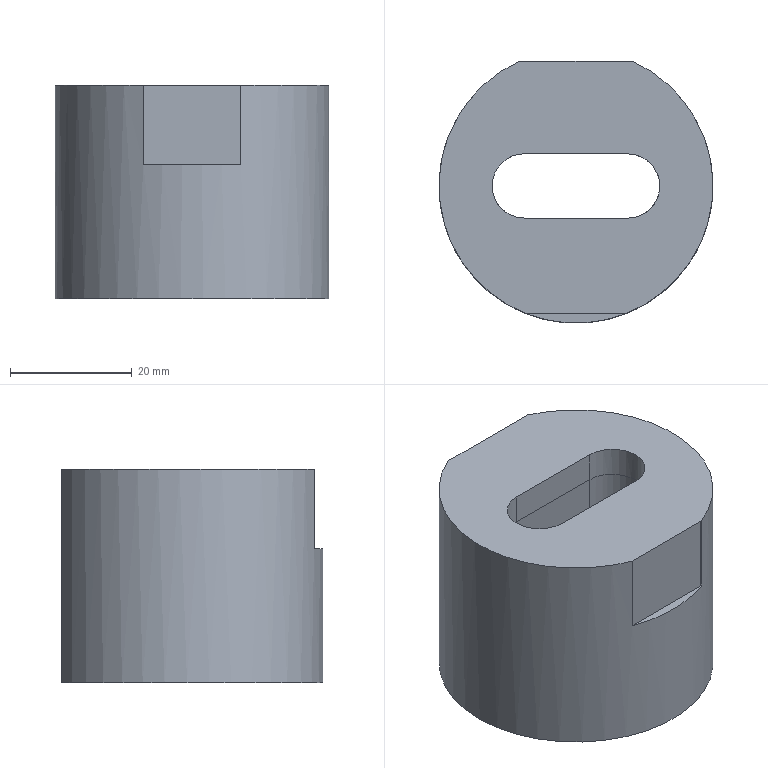Part | STEP file | lll_id322_x_t | 1 solid | 16 faces | box 45 x 43 x 35 mm | volume 44411 mm3 | plane 11 | spline 4 | cylinder 1 | commonest cylinder face diameters 45 x1
STEP:
#1=CARTESIAN_POINT('',(3410.226,-36.5,-35.));
#2=VERTEX_POINT('',#1);
#3=CARTESIAN_POINT('',(3428.774,-36.5,-35.));
#4=VERTEX_POINT('',#3);
#5=CARTESIAN_POINT('',(3419.5,-36.5,-35.));
#6=DIRECTION('',(1.,0.,0.));
#7=VECTOR('',#6,1.);
#8=LINE('',#5,#7);
#9=EDGE_CURVE('',#2,#4,#8,.T.);
#10=ORIENTED_EDGE('',*,*,#9,.T.);
#11=CARTESIAN_POINT('',(3419.5,-57.,-35.));
#12=DIRECTION('',(0.,0.,-1.));
#13=DIRECTION('',(-1.,0.,0.));
#14=AXIS2_PLACEMENT_3D('',#11,#12,#13);
#15=CIRCLE('',#14,22.5);
#16=EDGE_CURVE('',#4,#2,#15,.T.);
#17=ORIENTED_EDGE('',*,*,#16,.T.);
#18=EDGE_LOOP('',(#10,#17));
#19=FACE_BOUND('',#18,.T.);
#20=CARTESIAN_POINT('',(3411.,-63.071,-35.));
#21=VERTEX_POINT('',#20);
#22=CARTESIAN_POINT('',(3428.,-63.071,-35.));
#23=VERTEX_POINT('',#22);
#24=CARTESIAN_POINT('',(3419.5,-63.071,-35.));
#25=DIRECTION('',(1.,0.,0.));
#26=VECTOR('',#25,1.);
#27=LINE('',#24,#26);
#28=EDGE_CURVE('',#21,#23,#27,.T.);
#29=ORIENTED_EDGE('',*,*,#28,.T.);
#30=CARTESIAN_POINT('',(3428.,-50.929,-35.));
#31=VERTEX_POINT('',#30);
#32=CARTESIAN_POINT('',(3428.,-63.071,-35.));
#33=CARTESIAN_POINT('',(3428.,-63.071,-35.));
#34=CARTESIAN_POINT('',(3428.,-63.071,-35.));
#35=CARTESIAN_POINT('',(3429.609,-63.07,-35.));
#36=CARTESIAN_POINT('',(3431.162,-62.426,-35.));
#37=CARTESIAN_POINT('',(3433.432,-60.15,-35.));
#38=CARTESIAN_POINT('',(3434.072,-58.586,-35.));
#39=CARTESIAN_POINT('',(3434.069,-55.403,-35.));
#40=CARTESIAN_POINT('',(3433.419,-53.834,-35.));
#41=CARTESIAN_POINT('',(3431.167,-51.581,-35.));
#42=CARTESIAN_POINT('',(3429.612,-50.93,-35.));
#43=CARTESIAN_POINT('',(3428.,-50.929,-35.));
#44=B_SPLINE_CURVE_WITH_KNOTS('',3,(#32,#33,#34,#35,#36,#37,#38,#39,#40,#41,#42,#43),.UNSPECIFIED.,.F.,.F.,(4,2,2,2,2,4),(0.,0.00001007,0.25,0.5,0.75,1.),.UNSPECIFIED.);
#45=EDGE_CURVE('',#23,#31,#44,.T.);
#46=ORIENTED_EDGE('',*,*,#45,.T.);
#47=CARTESIAN_POINT('',(3411.,-50.929,-35.));
#48=VERTEX_POINT('',#47);
#49=CARTESIAN_POINT('',(3419.5,-50.929,-35.));
#50=DIRECTION('',(-1.,0.,0.));
#51=VECTOR('',#50,1.);
#52=LINE('',#49,#51);
#53=EDGE_CURVE('',#31,#48,#52,.T.);
#54=ORIENTED_EDGE('',*,*,#53,.T.);
#55=CARTESIAN_POINT('',(3411.,-50.929,-35.));
#56=CARTESIAN_POINT('',(3411.,-50.929,-35.));
#57=CARTESIAN_POINT('',(3411.,-50.929,-35.));
#58=CARTESIAN_POINT('',(3409.391,-50.93,-35.));
#59=CARTESIAN_POINT('',(3407.839,-51.574,-35.));
#60=CARTESIAN_POINT('',(3405.568,-53.849,-35.));
#61=CARTESIAN_POINT('',(3404.928,-55.413,-35.));
#62=CARTESIAN_POINT('',(3404.931,-58.597,-35.));
#63=CARTESIAN_POINT('',(3405.581,-60.165,-35.));
#64=CARTESIAN_POINT('',(3407.833,-62.418,-35.));
#65=CARTESIAN_POINT('',(3409.387,-63.07,-35.));
#66=CARTESIAN_POINT('',(3411.,-63.071,-35.));
#67=B_SPLINE_CURVE_WITH_KNOTS('',3,(#55,#56,#57,#58,#59,#60,#61,#62,#63,#64,#65,#66),.UNSPECIFIED.,.F.,.F.,(4,2,2,2,2,4),(0.,0.00001007,0.25,0.5,0.75,1.),.UNSPECIFIED.);
#68=EDGE_CURVE('',#48,#21,#67,.T.);
#69=ORIENTED_EDGE('',*,*,#68,.T.);
#70=EDGE_LOOP('',(#29,#46,#54,#69));
#71=FACE_BOUND('',#70,.T.);
#72=CARTESIAN_POINT('',(3419.5,-62.5,-35.));
#73=DIRECTION('',(0.,0.,-1.));
#74=DIRECTION('',(0.,1.,0.));
#75=AXIS2_PLACEMENT_3D('',#72,#73,#74);
#76=PLANE('',#75);
#77=ADVANCED_FACE('',(#19,#71),#76,.T.);
#78=CARTESIAN_POINT('',(3427.5,-78.,0.00001771));
#79=VERTEX_POINT('',#78);
#80=CARTESIAN_POINT('',(3411.5,-78.,0.00001771));
#81=VERTEX_POINT('',#80);
#82=CARTESIAN_POINT('',(3419.5,-78.,0.00001771));
#83=DIRECTION('',(-1.,0.,0.));
#84=VECTOR('',#83,1.);
#85=LINE('',#82,#84);
#86=EDGE_CURVE('',#79,#81,#85,.T.);
#87=ORIENTED_EDGE('',*,*,#86,.F.);
#88=CARTESIAN_POINT('',(3427.5,-78.03,0.00001771));
#89=VERTEX_POINT('',#88);
#90=CARTESIAN_POINT('',(3427.5,-86.,0.00001771));
#91=DIRECTION('',(0.,-1.,0.));
#92=VECTOR('',#91,1.);
#93=LINE('',#90,#92);
#94=EDGE_CURVE('',#79,#89,#93,.T.);
#95=ORIENTED_EDGE('',*,*,#94,.T.);
#96=CARTESIAN_POINT('',(3428.774,-36.5,0.00001771));
#97=VERTEX_POINT('',#96);
#98=CARTESIAN_POINT('',(3419.5,-57.,0.00001771));
#99=DIRECTION('',(0.,0.,-1.));
#100=DIRECTION('',(-1.,0.,0.));
#101=AXIS2_PLACEMENT_3D('',#98,#99,#100);
#102=CIRCLE('',#101,22.5);
#103=EDGE_CURVE('',#97,#89,#102,.T.);
#104=ORIENTED_EDGE('',*,*,#103,.F.);
#105=CARTESIAN_POINT('',(3410.226,-36.5,0.00001771));
#106=VERTEX_POINT('',#105);
#107=CARTESIAN_POINT('',(3419.5,-36.5,0.00001771));
#108=DIRECTION('',(-1.,0.,0.));
#109=VECTOR('',#108,1.);
#110=LINE('',#107,#109);
#111=EDGE_CURVE('',#97,#106,#110,.T.);
#112=ORIENTED_EDGE('',*,*,#111,.T.);
#113=CARTESIAN_POINT('',(3411.5,-78.03,0.00001771));
#114=VERTEX_POINT('',#113);
#115=CARTESIAN_POINT('',(3419.5,-57.,0.00001771));
#116=DIRECTION('',(0.,0.,-1.));
#117=DIRECTION('',(-1.,0.,0.));
#118=AXIS2_PLACEMENT_3D('',#115,#116,#117);
#119=CIRCLE('',#118,22.5);
#120=EDGE_CURVE('',#114,#106,#119,.T.);
#121=ORIENTED_EDGE('',*,*,#120,.F.);
#122=CARTESIAN_POINT('',(3411.5,-57.,0.00001771));
#123=DIRECTION('',(0.,-1.,0.));
#124=VECTOR('',#123,1.);
#125=LINE('',#122,#124);
#126=EDGE_CURVE('',#81,#114,#125,.T.);
#127=ORIENTED_EDGE('',*,*,#126,.F.);
#128=EDGE_LOOP('',(#87,#95,#104,#112,#121,#127));
#129=FACE_BOUND('',#128,.T.);
#130=CARTESIAN_POINT('',(3428.,-51.715,0.00001771));
#131=VERTEX_POINT('',#130);
#132=CARTESIAN_POINT('',(3428.,-62.285,0.00001771));
#133=VERTEX_POINT('',#132);
#134=CARTESIAN_POINT('',(3428.,-51.715,0.00001769));
#135=CARTESIAN_POINT('',(3429.386,-51.715,0.0000177));
#136=CARTESIAN_POINT('',(3430.756,-52.282,0.00001771));
#137=CARTESIAN_POINT('',(3432.718,-54.244,0.00001773));
#138=CARTESIAN_POINT('',(3433.285,-55.613,0.00001773));
#139=CARTESIAN_POINT('',(3433.285,-58.387,0.00001773));
#140=CARTESIAN_POINT('',(3432.718,-59.756,0.00001773));
#141=CARTESIAN_POINT('',(3431.247,-61.227,0.00001772));
#142=CARTESIAN_POINT('',(3430.659,-61.614,0.00001771));
#143=CARTESIAN_POINT('',(3429.701,-62.01,0.0000177));
#144=CARTESIAN_POINT('',(3429.37,-62.112,0.0000177));
#145=CARTESIAN_POINT('',(3428.692,-62.249,0.0000177));
#146=CARTESIAN_POINT('',(3428.33,-62.285,0.00001769));
#147=CARTESIAN_POINT('',(3428.,-62.285,0.00001769));
#148=B_SPLINE_CURVE_WITH_KNOTS('',3,(#134,#135,#136,#137,#138,#139,#140,#141,#142,#143,#144,#145,#146,#147),.UNSPECIFIED.,.F.,.F.,(4,2,2,2,2,2,4),(0.,0.25,0.5,0.75,0.875,0.9375,1.),.UNSPECIFIED.);
#149=EDGE_CURVE('',#131,#133,#148,.T.);
#150=ORIENTED_EDGE('',*,*,#149,.T.);
#151=CARTESIAN_POINT('',(3411.,-62.285,0.00001771));
#152=VERTEX_POINT('',#151);
#153=CARTESIAN_POINT('',(3419.5,-62.285,0.00001771));
#154=DIRECTION('',(-1.,0.,0.));
#155=VECTOR('',#154,1.);
#156=LINE('',#153,#155);
#157=EDGE_CURVE('',#133,#152,#156,.T.);
#158=ORIENTED_EDGE('',*,*,#157,.T.);
#159=CARTESIAN_POINT('',(3411.,-51.715,0.00001771));
#160=VERTEX_POINT('',#159);
#161=CARTESIAN_POINT('',(3411.,-62.285,0.00001772));
#162=CARTESIAN_POINT('',(3409.622,-62.285,0.00001771));
#163=CARTESIAN_POINT('',(3408.244,-61.719,0.0000177));
#164=CARTESIAN_POINT('',(3406.282,-59.756,0.00001769));
#165=CARTESIAN_POINT('',(3405.715,-58.387,0.00001768));
#166=CARTESIAN_POINT('',(3405.715,-55.613,0.00001768));
#167=CARTESIAN_POINT('',(3406.282,-54.244,0.00001769));
#168=CARTESIAN_POINT('',(3408.244,-52.282,0.0000177));
#169=CARTESIAN_POINT('',(3409.613,-51.715,0.00001771));
#170=CARTESIAN_POINT('',(3411.,-51.715,0.00001772));
#171=B_SPLINE_CURVE_WITH_KNOTS('',3,(#161,#162,#163,#164,#165,#166,#167,#168,#169,#170),.UNSPECIFIED.,.F.,.F.,(4,2,2,2,4),(0.,0.25,0.5,0.75,1.),.UNSPECIFIED.);
#172=EDGE_CURVE('',#152,#160,#171,.T.);
#173=ORIENTED_EDGE('',*,*,#172,.T.);
#174=CARTESIAN_POINT('',(3419.5,-51.715,0.00001771));
#175=DIRECTION('',(1.,0.,0.));
#176=VECTOR('',#175,1.);
#177=LINE('',#174,#176);
#178=EDGE_CURVE('',#160,#131,#177,.T.);
#179=ORIENTED_EDGE('',*,*,#178,.T.);
#180=EDGE_LOOP('',(#150,#158,#173,#179));
#181=FACE_BOUND('',#180,.T.);
#182=CARTESIAN_POINT('',(3419.5,-57.,0.00001771));
#183=DIRECTION('',(0.,0.,1.));
#184=DIRECTION('',(1.,0.,0.));
#185=AXIS2_PLACEMENT_3D('',#182,#183,#184);
#186=PLANE('',#185);
#187=ADVANCED_FACE('',(#129,#181),#186,.T.);
#188=ORIENTED_EDGE('',*,*,#103,.T.);
#189=CARTESIAN_POINT('',(3427.5,-78.03,-13.));
#190=VERTEX_POINT('',#189);
#191=CARTESIAN_POINT('',(3427.5,-78.03,-15.));
#192=DIRECTION('',(0.,0.,1.));
#193=VECTOR('',#192,1.);
#194=LINE('',#191,#193);
#195=EDGE_CURVE('',#190,#89,#194,.T.);
#196=ORIENTED_EDGE('',*,*,#195,.F.);
#197=CARTESIAN_POINT('',(3411.5,-78.03,-13.));
#198=VERTEX_POINT('',#197);
#199=CARTESIAN_POINT('',(3419.5,-57.,-13.));
#200=DIRECTION('',(0.,0.,1.));
#201=DIRECTION('',(-1.,0.,0.));
#202=AXIS2_PLACEMENT_3D('',#199,#200,#201);
#203=CIRCLE('',#202,22.5);
#204=EDGE_CURVE('',#198,#190,#203,.T.);
#205=ORIENTED_EDGE('',*,*,#204,.F.);
#206=CARTESIAN_POINT('',(3411.5,-78.03,-15.));
#207=DIRECTION('',(0.,0.,-1.));
#208=VECTOR('',#207,1.);
#209=LINE('',#206,#208);
#210=EDGE_CURVE('',#114,#198,#209,.T.);
#211=ORIENTED_EDGE('',*,*,#210,.F.);
#212=ORIENTED_EDGE('',*,*,#120,.T.);
#213=CARTESIAN_POINT('',(3410.226,-36.5,-15.));
#214=DIRECTION('',(0.,0.,-1.));
#215=VECTOR('',#214,1.);
#216=LINE('',#213,#215);
#217=EDGE_CURVE('',#106,#2,#216,.T.);
#218=ORIENTED_EDGE('',*,*,#217,.T.);
#219=ORIENTED_EDGE('',*,*,#16,.F.);
#220=CARTESIAN_POINT('',(3428.774,-36.5,-15.));
#221=DIRECTION('',(0.,0.,1.));
#222=VECTOR('',#221,1.);
#223=LINE('',#220,#222);
#224=EDGE_CURVE('',#4,#97,#223,.T.);
#225=ORIENTED_EDGE('',*,*,#224,.T.);
#226=EDGE_LOOP('',(#188,#196,#205,#211,#212,#218,#219,#225));
#227=FACE_OUTER_BOUND('',#226,.T.);
#228=CARTESIAN_POINT('',(3419.5,-57.,-15.));
#229=DIRECTION('',(0.,0.,-1.));
#230=DIRECTION('',(0.,-1.,0.));
#231=AXIS2_PLACEMENT_3D('',#228,#229,#230);
#232=CYLINDRICAL_SURFACE('',#231,22.5);
#233=ADVANCED_FACE('',(#227),#232,.T.);
#234=CARTESIAN_POINT('',(3428.,-62.285,-5.));
#235=VERTEX_POINT('',#234);
#236=CARTESIAN_POINT('',(3411.,-62.285,-5.));
#237=VERTEX_POINT('',#236);
#238=CARTESIAN_POINT('',(3428.,-62.285,-5.));
#239=DIRECTION('',(-1.,0.,0.));
#240=VECTOR('',#239,1.);
#241=LINE('',#238,#240);
#242=EDGE_CURVE('',#235,#237,#241,.T.);
#243=ORIENTED_EDGE('',*,*,#242,.T.);
#244=CARTESIAN_POINT('',(3411.,-62.285,2.5));
#245=DIRECTION('',(-0.000000008,0.,1.));
#246=VECTOR('',#245,1.);
#247=LINE('',#244,#246);
#248=EDGE_CURVE('',#237,#152,#247,.T.);
#249=ORIENTED_EDGE('',*,*,#248,.T.);
#250=ORIENTED_EDGE('',*,*,#157,.F.);
#251=CARTESIAN_POINT('',(3428.,-62.285,2.5));
#252=DIRECTION('',(-0.000000008,0.,1.));
#253=VECTOR('',#252,1.);
#254=LINE('',#251,#253);
#255=EDGE_CURVE('',#235,#133,#254,.T.);
#256=ORIENTED_EDGE('',*,*,#255,.F.);
#257=EDGE_LOOP('',(#243,#249,#250,#256));
#258=FACE_OUTER_BOUND('',#257,.T.);
#259=CARTESIAN_POINT('',(3433.,-62.285,2.5));
#260=DIRECTION('',(0.,1.,0.));
#261=DIRECTION('',(-1.,0.,-0.000000008));
#262=AXIS2_PLACEMENT_3D('',#259,#260,#261);
#263=PLANE('',#262);
#264=ADVANCED_FACE('',(#258),#263,.T.);
#265=CARTESIAN_POINT('',(3428.005,-62.285,-5.));
#266=VERTEX_POINT('',#265);
#267=CARTESIAN_POINT('',(3428.005,-62.285,-5.));
#268=CARTESIAN_POINT('',(3428.004,-62.285,-5.));
#269=CARTESIAN_POINT('',(3428.002,-62.285,-5.));
#270=CARTESIAN_POINT('',(3428.,-62.285,-5.));
#271=B_SPLINE_CURVE_WITH_KNOTS('',3,(#267,#268,#269,#270),.UNSPECIFIED.,.F.,.F.,(4,4),(0.,1.),.UNSPECIFIED.);
#272=EDGE_CURVE('',#266,#235,#271,.T.);
#273=ORIENTED_EDGE('',*,*,#272,.T.);
#274=ORIENTED_EDGE('',*,*,#255,.T.);
#275=ORIENTED_EDGE('',*,*,#149,.F.);
#276=CARTESIAN_POINT('',(3428.,-51.715,-5.));
#277=VERTEX_POINT('',#276);
#278=CARTESIAN_POINT('',(3428.,-51.715,2.5));
#279=DIRECTION('',(-0.000000008,0.,1.));
#280=VECTOR('',#279,1.);
#281=LINE('',#278,#280);
#282=EDGE_CURVE('',#277,#131,#281,.T.);
#283=ORIENTED_EDGE('',*,*,#282,.F.);
#284=CARTESIAN_POINT('',(3428.006,-51.715,-5.));
#285=VERTEX_POINT('',#284);
#286=CARTESIAN_POINT('',(3428.,-51.715,-5.));
#287=CARTESIAN_POINT('',(3428.002,-51.715,-5.));
#288=CARTESIAN_POINT('',(3428.004,-51.715,-5.));
#289=CARTESIAN_POINT('',(3428.006,-51.715,-5.));
#290=B_SPLINE_CURVE_WITH_KNOTS('',3,(#286,#287,#288,#289),.UNSPECIFIED.,.F.,.F.,(4,4),(0.,1.),.UNSPECIFIED.);
#291=EDGE_CURVE('',#277,#285,#290,.T.);
#292=ORIENTED_EDGE('',*,*,#291,.T.);
#293=CARTESIAN_POINT('',(3431.732,-53.258,-5.));
#294=VERTEX_POINT('',#293);
#295=CARTESIAN_POINT('',(3428.006,-51.715,-5.));
#296=CARTESIAN_POINT('',(3429.388,-51.717,-5.));
#297=CARTESIAN_POINT('',(3430.753,-52.282,-5.));
#298=CARTESIAN_POINT('',(3431.732,-53.258,-5.));
#299=B_SPLINE_CURVE_WITH_KNOTS('',3,(#295,#296,#297,#298),.UNSPECIFIED.,.F.,.F.,(4,4),(0.,1.),.UNSPECIFIED.);
#300=EDGE_CURVE('',#285,#294,#299,.T.);
#301=ORIENTED_EDGE('',*,*,#300,.T.);
#302=CARTESIAN_POINT('',(3433.285,-56.998,-5.));
#303=VERTEX_POINT('',#302);
#304=CARTESIAN_POINT('',(3431.732,-53.258,-5.));
#305=CARTESIAN_POINT('',(3431.896,-53.421,-5.));
#306=CARTESIAN_POINT('',(3432.133,-53.675,-5.012));
#307=CARTESIAN_POINT('',(3432.645,-54.445,-5.058));
#308=CARTESIAN_POINT('',(3432.789,-54.762,-5.07));
#309=CARTESIAN_POINT('',(3432.965,-55.188,-5.07));
#310=CARTESIAN_POINT('',(3433.089,-55.513,-5.059));
#311=CARTESIAN_POINT('',(3433.272,-56.419,-5.012));
#312=CARTESIAN_POINT('',(3433.285,-56.768,-5.));
#313=CARTESIAN_POINT('',(3433.285,-56.998,-5.));
#314=B_SPLINE_CURVE_WITH_KNOTS('',3,(#304,#305,#306,#307,#308,#309,#310,#311,#312,#313),.UNSPECIFIED.,.F.,.F.,(4,2,2,2,4),(0.,0.25,0.5,0.75,1.),.UNSPECIFIED.);
#315=EDGE_CURVE('',#294,#303,#314,.T.);
#316=ORIENTED_EDGE('',*,*,#315,.T.);
#317=CARTESIAN_POINT('',(3433.045,-58.562,-5.));
#318=VERTEX_POINT('',#317);
#319=CARTESIAN_POINT('',(3433.285,-56.998,-5.001));
#320=CARTESIAN_POINT('',(3433.285,-56.998,-5.001));
#321=CARTESIAN_POINT('',(3433.285,-56.999,-5.001));
#322=CARTESIAN_POINT('',(3433.285,-57.53,-5.001));
#323=CARTESIAN_POINT('',(3433.202,-58.058,-5.001));
#324=CARTESIAN_POINT('',(3433.045,-58.562,-5.001));
#325=B_SPLINE_CURVE_WITH_KNOTS('',3,(#319,#320,#321,#322,#323,#324),.UNSPECIFIED.,.F.,.F.,(4,2,4),(0.,0.001523,1.),.UNSPECIFIED.);
#326=EDGE_CURVE('',#303,#318,#325,.T.);
#327=ORIENTED_EDGE('',*,*,#326,.T.);
#328=CARTESIAN_POINT('',(3431.742,-60.732,-5.));
#329=VERTEX_POINT('',#328);
#330=CARTESIAN_POINT('',(3433.045,-58.562,-5.));
#331=CARTESIAN_POINT('',(3432.792,-59.375,-5.));
#332=CARTESIAN_POINT('',(3432.346,-60.127,-5.));
#333=CARTESIAN_POINT('',(3431.742,-60.732,-5.));
#334=B_SPLINE_CURVE_WITH_KNOTS('',3,(#330,#331,#332,#333),.UNSPECIFIED.,.F.,.F.,(4,4),(0.,1.),.UNSPECIFIED.);
#335=EDGE_CURVE('',#318,#329,#334,.T.);
#336=ORIENTED_EDGE('',*,*,#335,.T.);
#337=CARTESIAN_POINT('',(3431.742,-60.732,-5.));
#338=CARTESIAN_POINT('',(3431.741,-60.734,-5.));
#339=CARTESIAN_POINT('',(3431.739,-60.735,-5.));
#340=CARTESIAN_POINT('',(3431.247,-61.227,-5.));
#341=CARTESIAN_POINT('',(3430.659,-61.614,-5.));
#342=CARTESIAN_POINT('',(3429.701,-62.01,-5.));
#343=CARTESIAN_POINT('',(3429.37,-62.112,-5.));
#344=CARTESIAN_POINT('',(3428.694,-62.249,-5.));
#345=CARTESIAN_POINT('',(3428.334,-62.285,-5.));
#346=CARTESIAN_POINT('',(3428.005,-62.285,-5.));
#347=B_SPLINE_CURVE_WITH_KNOTS('',3,(#337,#338,#339,#340,#341,#342,#343,#344,#345,#346),.UNSPECIFIED.,.F.,.F.,(4,2,2,2,4),(0.,0.001784,0.5016,0.7515,1.),.UNSPECIFIED.);
#348=EDGE_CURVE('',#329,#266,#347,.T.);
#349=ORIENTED_EDGE('',*,*,#348,.T.);
#350=EDGE_LOOP('',(#273,#274,#275,#283,#292,#301,#316,#327,#336,#349));
#351=FACE_OUTER_BOUND('',#350,.T.);
#352=CARTESIAN_POINT('',(3428.,-51.715,-5.106));
#353=CARTESIAN_POINT('',(3428.,-51.715,0.00001771));
#354=CARTESIAN_POINT('',(3429.386,-51.715,-5.106));
#355=CARTESIAN_POINT('',(3429.386,-51.715,0.00001772));
#356=CARTESIAN_POINT('',(3430.756,-52.282,-5.106));
#357=CARTESIAN_POINT('',(3430.756,-52.282,0.00001773));
#358=CARTESIAN_POINT('',(3432.718,-54.244,-5.106));
#359=CARTESIAN_POINT('',(3432.718,-54.244,0.00001775));
#360=CARTESIAN_POINT('',(3433.285,-55.613,-5.106));
#361=CARTESIAN_POINT('',(3433.285,-55.613,0.00001775));
#362=CARTESIAN_POINT('',(3433.285,-58.387,-5.106));
#363=CARTESIAN_POINT('',(3433.285,-58.387,0.00001775));
#364=CARTESIAN_POINT('',(3432.718,-59.756,-5.106));
#365=CARTESIAN_POINT('',(3432.718,-59.756,0.00001775));
#366=CARTESIAN_POINT('',(3431.247,-61.227,-5.106));
#367=CARTESIAN_POINT('',(3431.247,-61.227,0.00001774));
#368=CARTESIAN_POINT('',(3430.659,-61.614,-5.106));
#369=CARTESIAN_POINT('',(3430.659,-61.614,0.00001773));
#370=CARTESIAN_POINT('',(3429.701,-62.01,-5.106));
#371=CARTESIAN_POINT('',(3429.701,-62.01,0.00001772));
#372=CARTESIAN_POINT('',(3429.37,-62.112,-5.106));
#373=CARTESIAN_POINT('',(3429.37,-62.112,0.00001772));
#374=CARTESIAN_POINT('',(3428.692,-62.249,-5.106));
#375=CARTESIAN_POINT('',(3428.692,-62.249,0.00001772));
#376=CARTESIAN_POINT('',(3428.33,-62.285,-5.106));
#377=CARTESIAN_POINT('',(3428.33,-62.285,0.00001771));
#378=CARTESIAN_POINT('',(3428.,-62.285,-5.106));
#379=CARTESIAN_POINT('',(3428.,-62.285,0.00001771));
#380=B_SPLINE_SURFACE_WITH_KNOTS('',3,1,((#352,#353),(#354,#355),(#356,#357),(#358,#359),(#360,#361),(#362,#363),(#364,#365),(#366,#367),(#368,#369),(#370,#371),(#372,#373),(#374,#375),(#376,#377),(#378,#379)),.UNSPECIFIED.,.F.,.F.,.F.,(4,2,2,2,2,2,4),(2,2),(0.,0.25,0.5,0.75,0.875,0.9375,1.),(0.,1.),.UNSPECIFIED.);
#381=ADVANCED_FACE('',(#351),#380,.T.);
#382=CARTESIAN_POINT('',(3411.,-51.715,-5.));
#383=VERTEX_POINT('',#382);
#384=CARTESIAN_POINT('',(3411.,-51.715,-5.));
#385=DIRECTION('',(1.,0.,0.));
#386=VECTOR('',#385,1.);
#387=LINE('',#384,#386);
#388=EDGE_CURVE('',#383,#277,#387,.T.);
#389=ORIENTED_EDGE('',*,*,#388,.T.);
#390=ORIENTED_EDGE('',*,*,#282,.T.);
#391=ORIENTED_EDGE('',*,*,#178,.F.);
#392=CARTESIAN_POINT('',(3411.,-51.715,2.5));
#393=DIRECTION('',(-0.000000008,0.,1.));
#394=VECTOR('',#393,1.);
#395=LINE('',#392,#394);
#396=EDGE_CURVE('',#383,#160,#395,.T.);
#397=ORIENTED_EDGE('',*,*,#396,.F.);
#398=EDGE_LOOP('',(#389,#390,#391,#397));
#399=FACE_OUTER_BOUND('',#398,.T.);
#400=CARTESIAN_POINT('',(3433.,-51.715,2.5));
#401=DIRECTION('',(0.,-1.,0.));
#402=DIRECTION('',(1.,0.,0.000000008));
#403=AXIS2_PLACEMENT_3D('',#400,#401,#402);
#404=PLANE('',#403);
#405=ADVANCED_FACE('',(#399),#404,.T.);
#406=CARTESIAN_POINT('',(3410.995,-51.715,-5.));
#407=VERTEX_POINT('',#406);
#408=CARTESIAN_POINT('',(3410.995,-51.715,-5.));
#409=CARTESIAN_POINT('',(3410.996,-51.715,-5.));
#410=CARTESIAN_POINT('',(3410.998,-51.715,-5.));
#411=CARTESIAN_POINT('',(3411.,-51.715,-5.));
#412=B_SPLINE_CURVE_WITH_KNOTS('',3,(#408,#409,#410,#411),.UNSPECIFIED.,.F.,.F.,(4,4),(0.,1.),.UNSPECIFIED.);
#413=EDGE_CURVE('',#407,#383,#412,.T.);
#414=ORIENTED_EDGE('',*,*,#413,.T.);
#415=ORIENTED_EDGE('',*,*,#396,.T.);
#416=ORIENTED_EDGE('',*,*,#172,.F.);
#417=ORIENTED_EDGE('',*,*,#248,.F.);
#418=CARTESIAN_POINT('',(3410.994,-62.285,-5.));
#419=VERTEX_POINT('',#418);
#420=CARTESIAN_POINT('',(3411.,-62.285,-5.));
#421=CARTESIAN_POINT('',(3410.998,-62.285,-5.));
#422=CARTESIAN_POINT('',(3410.996,-62.285,-5.));
#423=CARTESIAN_POINT('',(3410.994,-62.285,-5.));
#424=B_SPLINE_CURVE_WITH_KNOTS('',3,(#420,#421,#422,#423),.UNSPECIFIED.,.F.,.F.,(4,4),(0.,1.),.UNSPECIFIED.);
#425=EDGE_CURVE('',#237,#419,#424,.T.);
#426=ORIENTED_EDGE('',*,*,#425,.T.);
#427=CARTESIAN_POINT('',(3407.26,-60.734,-5.));
#428=VERTEX_POINT('',#427);
#429=CARTESIAN_POINT('',(3410.994,-62.285,-5.));
#430=CARTESIAN_POINT('',(3409.618,-62.283,-5.));
#431=CARTESIAN_POINT('',(3408.243,-61.717,-5.));
#432=CARTESIAN_POINT('',(3407.262,-60.736,-5.));
#433=CARTESIAN_POINT('',(3407.261,-60.735,-5.));
#434=CARTESIAN_POINT('',(3407.26,-60.734,-5.));
#435=B_SPLINE_CURVE_WITH_KNOTS('',3,(#429,#430,#431,#432,#433,#434),.UNSPECIFIED.,.F.,.F.,(4,2,4),(0.,0.9989,1.),.UNSPECIFIED.);
#436=EDGE_CURVE('',#419,#428,#435,.T.);
#437=ORIENTED_EDGE('',*,*,#436,.T.);
#438=CARTESIAN_POINT('',(3405.715,-57.002,-5.));
#439=VERTEX_POINT('',#438);
#440=CARTESIAN_POINT('',(3407.26,-60.734,-5.));
#441=CARTESIAN_POINT('',(3407.098,-60.572,-5.));
#442=CARTESIAN_POINT('',(3406.861,-60.316,-5.012));
#443=CARTESIAN_POINT('',(3406.352,-59.549,-5.059));
#444=CARTESIAN_POINT('',(3406.208,-59.232,-5.071));
#445=CARTESIAN_POINT('',(3406.033,-58.808,-5.071));
#446=CARTESIAN_POINT('',(3405.91,-58.483,-5.059));
#447=CARTESIAN_POINT('',(3405.728,-57.58,-5.012));
#448=CARTESIAN_POINT('',(3405.715,-57.232,-5.));
#449=CARTESIAN_POINT('',(3405.715,-57.002,-5.));
#450=B_SPLINE_CURVE_WITH_KNOTS('',3,(#440,#441,#442,#443,#444,#445,#446,#447,#448,#449),.UNSPECIFIED.,.F.,.F.,(4,2,2,2,4),(0.,0.25,0.5,0.75,1.),.UNSPECIFIED.);
#451=EDGE_CURVE('',#428,#439,#450,.T.);
#452=ORIENTED_EDGE('',*,*,#451,.T.);
#453=CARTESIAN_POINT('',(3406.035,-55.202,-5.));
#454=VERTEX_POINT('',#453);
#455=CARTESIAN_POINT('',(3405.715,-57.002,-5.001));
#456=CARTESIAN_POINT('',(3405.715,-57.002,-5.001));
#457=CARTESIAN_POINT('',(3405.715,-57.001,-5.001));
#458=CARTESIAN_POINT('',(3405.715,-56.387,-5.001));
#459=CARTESIAN_POINT('',(3405.826,-55.776,-5.001));
#460=CARTESIAN_POINT('',(3406.035,-55.202,-5.001));
#461=B_SPLINE_CURVE_WITH_KNOTS('',3,(#455,#456,#457,#458,#459,#460),.UNSPECIFIED.,.F.,.F.,(4,2,4),(0.,0.001199,1.),.UNSPECIFIED.);
#462=EDGE_CURVE('',#439,#454,#461,.T.);
#463=ORIENTED_EDGE('',*,*,#462,.T.);
#464=CARTESIAN_POINT('',(3407.258,-53.268,-5.));
#465=VERTEX_POINT('',#464);
#466=CARTESIAN_POINT('',(3406.035,-55.202,-5.));
#467=CARTESIAN_POINT('',(3406.297,-54.48,-5.));
#468=CARTESIAN_POINT('',(3406.713,-53.814,-5.));
#469=CARTESIAN_POINT('',(3407.258,-53.268,-5.));
#470=B_SPLINE_CURVE_WITH_KNOTS('',3,(#466,#467,#468,#469),.UNSPECIFIED.,.F.,.F.,(4,4),(0.,1.),.UNSPECIFIED.);
#471=EDGE_CURVE('',#454,#465,#470,.T.);
#472=ORIENTED_EDGE('',*,*,#471,.T.);
#473=CARTESIAN_POINT('',(3407.258,-53.268,-5.));
#474=CARTESIAN_POINT('',(3407.259,-53.266,-5.));
#475=CARTESIAN_POINT('',(3407.261,-53.265,-5.));
#476=CARTESIAN_POINT('',(3408.242,-52.283,-5.));
#477=CARTESIAN_POINT('',(3409.61,-51.717,-5.));
#478=CARTESIAN_POINT('',(3410.995,-51.715,-5.));
#479=B_SPLINE_CURVE_WITH_KNOTS('',3,(#473,#474,#475,#476,#477,#478),.UNSPECIFIED.,.F.,.F.,(4,2,4),(0.,0.001796,1.),.UNSPECIFIED.);
#480=EDGE_CURVE('',#465,#407,#479,.T.);
#481=ORIENTED_EDGE('',*,*,#480,.T.);
#482=EDGE_LOOP('',(#414,#415,#416,#417,#426,#437,#452,#463,#472,#481));
#483=FACE_OUTER_BOUND('',#482,.T.);
#484=CARTESIAN_POINT('',(3411.,-62.285,-5.108));
#485=CARTESIAN_POINT('',(3411.,-62.285,0.00001773));
#486=CARTESIAN_POINT('',(3409.622,-62.285,-5.108));
#487=CARTESIAN_POINT('',(3409.622,-62.285,0.00001772));
#488=CARTESIAN_POINT('',(3408.244,-61.719,-5.108));
#489=CARTESIAN_POINT('',(3408.244,-61.719,0.00001771));
#490=CARTESIAN_POINT('',(3406.282,-59.756,-5.108));
#491=CARTESIAN_POINT('',(3406.282,-59.756,0.0000177));
#492=CARTESIAN_POINT('',(3405.715,-58.387,-5.108));
#493=CARTESIAN_POINT('',(3405.715,-58.387,0.00001769));
#494=CARTESIAN_POINT('',(3405.715,-55.613,-5.108));
#495=CARTESIAN_POINT('',(3405.715,-55.613,0.00001769));
#496=CARTESIAN_POINT('',(3406.282,-54.244,-5.108));
#497=CARTESIAN_POINT('',(3406.282,-54.244,0.0000177));
#498=CARTESIAN_POINT('',(3408.244,-52.282,-5.108));
#499=CARTESIAN_POINT('',(3408.244,-52.282,0.00001771));
#500=CARTESIAN_POINT('',(3409.613,-51.715,-5.108));
#501=CARTESIAN_POINT('',(3409.613,-51.715,0.00001772));
#502=CARTESIAN_POINT('',(3411.,-51.715,-5.108));
#503=CARTESIAN_POINT('',(3411.,-51.715,0.00001773));
#504=B_SPLINE_SURFACE_WITH_KNOTS('',3,1,((#484,#485),(#486,#487),(#488,#489),(#490,#491),(#492,#493),(#494,#495),(#496,#497),(#498,#499),(#500,#501),(#502,#503)),.UNSPECIFIED.,.F.,.F.,.F.,(4,2,2,2,4),(2,2),(0.,0.25,0.5,0.75,1.),(0.,1.),.UNSPECIFIED.);
#505=ADVANCED_FACE('',(#483),#504,.T.);
#506=ORIENTED_EDGE('',*,*,#224,.F.);
#507=ORIENTED_EDGE('',*,*,#9,.F.);
#508=ORIENTED_EDGE('',*,*,#217,.F.);
#509=ORIENTED_EDGE('',*,*,#111,.F.);
#510=EDGE_LOOP('',(#506,#507,#508,#509));
#511=FACE_OUTER_BOUND('',#510,.T.);
#512=CARTESIAN_POINT('',(3419.5,-36.5,-32.5));
#513=DIRECTION('',(0.,1.,0.));
#514=DIRECTION('',(0.,0.,-1.));
#515=AXIS2_PLACEMENT_3D('',#512,#513,#514);
#516=PLANE('',#515);
#517=ADVANCED_FACE('',(#511),#516,.T.);
#518=CARTESIAN_POINT('',(3428.,-62.285,-5.));
#519=DIRECTION('',(0.,-0.02618,-0.9997));
#520=VECTOR('',#519,1.);
#521=LINE('',#518,#520);
#522=EDGE_CURVE('',#235,#23,#521,.T.);
#523=ORIENTED_EDGE('',*,*,#522,.F.);
#524=ORIENTED_EDGE('',*,*,#272,.F.);
#525=ORIENTED_EDGE('',*,*,#348,.F.);
#526=ORIENTED_EDGE('',*,*,#335,.F.);
#527=ORIENTED_EDGE('',*,*,#326,.F.);
#528=ORIENTED_EDGE('',*,*,#315,.F.);
#529=ORIENTED_EDGE('',*,*,#300,.F.);
#530=ORIENTED_EDGE('',*,*,#291,.F.);
#531=CARTESIAN_POINT('',(3428.,-51.715,-5.));
#532=DIRECTION('',(0.000006156,0.02618,-0.9997));
#533=VECTOR('',#532,1.);
#534=LINE('',#531,#533);
#535=EDGE_CURVE('',#277,#31,#534,.T.);
#536=ORIENTED_EDGE('',*,*,#535,.T.);
#537=ORIENTED_EDGE('',*,*,#45,.F.);
#538=EDGE_LOOP('',(#523,#524,#525,#526,#527,#528,#529,#530,#536,#537));
#539=FACE_OUTER_BOUND('',#538,.T.);
#540=CARTESIAN_POINT('',(3428.,-51.715,-5.));
#541=CARTESIAN_POINT('',(3429.396,-51.715,-5.));
#542=CARTESIAN_POINT('',(3430.763,-52.289,-5.));
#543=CARTESIAN_POINT('',(3432.711,-54.237,-5.));
#544=CARTESIAN_POINT('',(3433.284,-55.619,-5.));
#545=CARTESIAN_POINT('',(3433.286,-58.371,-5.));
#546=CARTESIAN_POINT('',(3432.725,-59.747,-5.));
#547=CARTESIAN_POINT('',(3430.757,-61.72,-5.));
#548=CARTESIAN_POINT('',(3429.396,-62.285,-5.));
#549=CARTESIAN_POINT('',(3427.944,-62.285,-5.));
#550=CARTESIAN_POINT('',(3427.888,-62.285,-5.));
#551=CARTESIAN_POINT('',(3427.833,-62.285,-5.));
#552=CARTESIAN_POINT('',(3428.,-50.615,-47.));
#553=CARTESIAN_POINT('',(3429.699,-50.616,-47.));
#554=CARTESIAN_POINT('',(3431.328,-51.298,-47.));
#555=CARTESIAN_POINT('',(3433.702,-53.673,-47.));
#556=CARTESIAN_POINT('',(3434.383,-55.316,-47.));
#557=CARTESIAN_POINT('',(3434.386,-58.672,-47.));
#558=CARTESIAN_POINT('',(3433.715,-60.312,-47.));
#559=CARTESIAN_POINT('',(3431.324,-62.709,-47.));
#560=CARTESIAN_POINT('',(3429.694,-63.384,-47.));
#561=CARTESIAN_POINT('',(3427.933,-63.385,-47.));
#562=CARTESIAN_POINT('',(3427.865,-63.385,-47.));
#563=CARTESIAN_POINT('',(3427.797,-63.385,-47.));
#564=B_SPLINE_SURFACE_WITH_KNOTS('',1,3,((#540,#541,#542,#543,#544,#545,#546,#547,#548,#549,#550,#551),(#552,#553,#554,#555,#556,#557,#558,#559,#560,#561,#562,#563)),.UNSPECIFIED.,.F.,.F.,.F.,(2,2),(4,2,2,2,2,4),(0.,1.),(0.,0.2475,0.495,0.7426,0.9901,1.),.UNSPECIFIED.);
#565=ADVANCED_FACE('',(#539),#564,.T.);
#566=CARTESIAN_POINT('',(3411.,-62.285,-5.));
#567=DIRECTION('',(-0.000006179,-0.02618,-0.9997));
#568=VECTOR('',#567,1.);
#569=LINE('',#566,#568);
#570=EDGE_CURVE('',#237,#21,#569,.T.);
#571=ORIENTED_EDGE('',*,*,#570,.F.);
#572=ORIENTED_EDGE('',*,*,#242,.F.);
#573=ORIENTED_EDGE('',*,*,#522,.T.);
#574=ORIENTED_EDGE('',*,*,#28,.F.);
#575=EDGE_LOOP('',(#571,#572,#573,#574));
#576=FACE_OUTER_BOUND('',#575,.T.);
#577=CARTESIAN_POINT('',(3428.,-62.285,-5.));
#578=DIRECTION('',(0.,0.9997,-0.02618));
#579=DIRECTION('',(0.,0.02618,0.9997));
#580=AXIS2_PLACEMENT_3D('',#577,#578,#579);
#581=PLANE('',#580);
#582=ADVANCED_FACE('',(#576),#581,.T.);
#583=CARTESIAN_POINT('',(3411.,-51.715,-5.));
#584=DIRECTION('',(0.,0.02618,-0.9997));
#585=VECTOR('',#584,1.);
#586=LINE('',#583,#585);
#587=EDGE_CURVE('',#383,#48,#586,.T.);
#588=ORIENTED_EDGE('',*,*,#587,.F.);
#589=ORIENTED_EDGE('',*,*,#413,.F.);
#590=ORIENTED_EDGE('',*,*,#480,.F.);
#591=ORIENTED_EDGE('',*,*,#471,.F.);
#592=ORIENTED_EDGE('',*,*,#462,.F.);
#593=ORIENTED_EDGE('',*,*,#451,.F.);
#594=ORIENTED_EDGE('',*,*,#436,.F.);
#595=ORIENTED_EDGE('',*,*,#425,.F.);
#596=ORIENTED_EDGE('',*,*,#570,.T.);
#597=ORIENTED_EDGE('',*,*,#68,.F.);
#598=EDGE_LOOP('',(#588,#589,#590,#591,#592,#593,#594,#595,#596,#597));
#599=FACE_OUTER_BOUND('',#598,.T.);
#600=CARTESIAN_POINT('',(3411.,-62.285,-5.));
#601=CARTESIAN_POINT('',(3409.603,-62.285,-5.));
#602=CARTESIAN_POINT('',(3408.236,-61.71,-5.));
#603=CARTESIAN_POINT('',(3406.289,-59.762,-5.));
#604=CARTESIAN_POINT('',(3405.716,-58.38,-5.));
#605=CARTESIAN_POINT('',(3405.714,-55.629,-5.));
#606=CARTESIAN_POINT('',(3406.275,-54.253,-5.));
#607=CARTESIAN_POINT('',(3408.243,-52.28,-5.));
#608=CARTESIAN_POINT('',(3409.604,-51.715,-5.));
#609=CARTESIAN_POINT('',(3411.056,-51.715,-5.));
#610=CARTESIAN_POINT('',(3411.112,-51.715,-5.));
#611=CARTESIAN_POINT('',(3411.167,-51.715,-5.));
#612=CARTESIAN_POINT('',(3411.,-63.385,-47.));
#613=CARTESIAN_POINT('',(3409.301,-63.384,-47.));
#614=CARTESIAN_POINT('',(3407.671,-62.701,-47.));
#615=CARTESIAN_POINT('',(3405.297,-60.327,-47.));
#616=CARTESIAN_POINT('',(3404.617,-58.683,-47.));
#617=CARTESIAN_POINT('',(3404.614,-55.327,-47.));
#618=CARTESIAN_POINT('',(3405.285,-53.688,-47.));
#619=CARTESIAN_POINT('',(3407.677,-51.291,-47.));
#620=CARTESIAN_POINT('',(3409.306,-50.616,-47.));
#621=CARTESIAN_POINT('',(3411.067,-50.615,-47.));
#622=CARTESIAN_POINT('',(3411.135,-50.615,-47.));
#623=CARTESIAN_POINT('',(3411.203,-50.615,-47.));
#624=B_SPLINE_SURFACE_WITH_KNOTS('',1,3,((#600,#601,#602,#603,#604,#605,#606,#607,#608,#609,#610,#611),(#612,#613,#614,#615,#616,#617,#618,#619,#620,#621,#622,#623)),.UNSPECIFIED.,.F.,.F.,.F.,(2,2),(4,2,2,2,2,4),(0.,1.),(0.,0.2475,0.495,0.7426,0.9901,1.),.UNSPECIFIED.);
#625=ADVANCED_FACE('',(#599),#624,.T.);
#626=ORIENTED_EDGE('',*,*,#535,.F.);
#627=ORIENTED_EDGE('',*,*,#388,.F.);
#628=ORIENTED_EDGE('',*,*,#587,.T.);
#629=ORIENTED_EDGE('',*,*,#53,.F.);
#630=EDGE_LOOP('',(#626,#627,#628,#629));
#631=FACE_OUTER_BOUND('',#630,.T.);
#632=CARTESIAN_POINT('',(3411.,-51.715,-5.));
#633=DIRECTION('',(0.,-0.9997,-0.02618));
#634=DIRECTION('',(0.,0.02618,-0.9997));
#635=AXIS2_PLACEMENT_3D('',#632,#633,#634);
#636=PLANE('',#635);
#637=ADVANCED_FACE('',(#631),#636,.T.);
#638=ORIENTED_EDGE('',*,*,#94,.F.);
#639=CARTESIAN_POINT('',(3427.5,-78.,-13.));
#640=VERTEX_POINT('',#639);
#641=CARTESIAN_POINT('',(3427.5,-78.,-1.));
#642=DIRECTION('',(0.,0.,-1.));
#643=VECTOR('',#642,1.);
#644=LINE('',#641,#643);
#645=EDGE_CURVE('',#79,#640,#644,.T.);
#646=ORIENTED_EDGE('',*,*,#645,.T.);
#647=CARTESIAN_POINT('',(3427.5,-86.,-13.));
#648=DIRECTION('',(0.,-1.,0.));
#649=VECTOR('',#648,1.);
#650=LINE('',#647,#649);
#651=EDGE_CURVE('',#640,#190,#650,.T.);
#652=ORIENTED_EDGE('',*,*,#651,.T.);
#653=ORIENTED_EDGE('',*,*,#195,.T.);
#654=EDGE_LOOP('',(#638,#646,#652,#653));
#655=FACE_OUTER_BOUND('',#654,.T.);
#656=CARTESIAN_POINT('',(3427.5,-86.,-1.));
#657=DIRECTION('',(1.,0.,0.));
#658=DIRECTION('',(0.,0.,1.));
#659=AXIS2_PLACEMENT_3D('',#656,#657,#658);
#660=PLANE('',#659);
#661=ADVANCED_FACE('',(#655),#660,.F.);
#662=ORIENTED_EDGE('',*,*,#204,.T.);
#663=ORIENTED_EDGE('',*,*,#651,.F.);
#664=CARTESIAN_POINT('',(3411.5,-78.,-13.));
#665=VERTEX_POINT('',#664);
#666=CARTESIAN_POINT('',(3419.5,-78.,-13.));
#667=DIRECTION('',(1.,0.,0.));
#668=VECTOR('',#667,1.);
#669=LINE('',#666,#668);
#670=EDGE_CURVE('',#665,#640,#669,.T.);
#671=ORIENTED_EDGE('',*,*,#670,.F.);
#672=CARTESIAN_POINT('',(3411.5,-86.,-13.));
#673=DIRECTION('',(0.,1.,0.));
#674=VECTOR('',#673,1.);
#675=LINE('',#672,#674);
#676=EDGE_CURVE('',#198,#665,#675,.T.);
#677=ORIENTED_EDGE('',*,*,#676,.F.);
#678=EDGE_LOOP('',(#662,#663,#671,#677));
#679=FACE_OUTER_BOUND('',#678,.T.);
#680=CARTESIAN_POINT('',(3419.5,-86.,-13.));
#681=DIRECTION('',(0.,0.,-1.));
#682=DIRECTION('',(0.,1.,0.));
#683=AXIS2_PLACEMENT_3D('',#680,#681,#682);
#684=PLANE('',#683);
#685=ADVANCED_FACE('',(#679),#684,.F.);
#686=CARTESIAN_POINT('',(3411.5,-78.,-1.));
#687=DIRECTION('',(0.,0.,-1.));
#688=VECTOR('',#687,1.);
#689=LINE('',#686,#688);
#690=EDGE_CURVE('',#81,#665,#689,.T.);
#691=ORIENTED_EDGE('',*,*,#690,.F.);
#692=ORIENTED_EDGE('',*,*,#126,.T.);
#693=ORIENTED_EDGE('',*,*,#210,.T.);
#694=ORIENTED_EDGE('',*,*,#676,.T.);
#695=EDGE_LOOP('',(#691,#692,#693,#694));
#696=FACE_OUTER_BOUND('',#695,.T.);
#697=CARTESIAN_POINT('',(3411.5,-86.,-1.));
#698=DIRECTION('',(-1.,0.,0.));
#699=DIRECTION('',(0.,0.,-1.));
#700=AXIS2_PLACEMENT_3D('',#697,#698,#699);
#701=PLANE('',#700);
#702=ADVANCED_FACE('',(#696),#701,.F.);
#703=ORIENTED_EDGE('',*,*,#645,.F.);
#704=ORIENTED_EDGE('',*,*,#86,.T.);
#705=ORIENTED_EDGE('',*,*,#690,.T.);
#706=ORIENTED_EDGE('',*,*,#670,.T.);
#707=EDGE_LOOP('',(#703,#704,#705,#706));
#708=FACE_OUTER_BOUND('',#707,.T.);
#709=CARTESIAN_POINT('',(3419.5,-78.,-1.));
#710=DIRECTION('',(0.,1.,0.));
#711=DIRECTION('',(0.,0.,1.));
#712=AXIS2_PLACEMENT_3D('',#709,#710,#711);
#713=PLANE('',#712);
#714=ADVANCED_FACE('',(#708),#713,.F.);
#715=CLOSED_SHELL('',(#77,#187,#233,#264,#381,#405,#505,#517,#565,#582,#625,#637,#661,#685,#702,#714));
#716=MANIFOLD_SOLID_BREP('',#715);
#717=(LENGTH_UNIT()NAMED_UNIT(*)SI_UNIT(.MILLI.,.METRE.));
#718=UNCERTAINTY_MEASURE_WITH_UNIT(LENGTH_MEASURE(0.0508),#717,'','');
#719=(NAMED_UNIT(*)PLANE_ANGLE_UNIT()SI_UNIT($,.RADIAN.));
#720=PLANE_ANGLE_MEASURE_WITH_UNIT(PLANE_ANGLE_MEASURE(0.01745),#719);
#721=DIMENSIONAL_EXPONENTS(0.,0.,0.,0.,0.,0.,0.);
#722=(CONVERSION_BASED_UNIT('DEGREE',#720)NAMED_UNIT(#721)PLANE_ANGLE_UNIT());
#723=(NAMED_UNIT(*)SI_UNIT($,.STERADIAN.)SOLID_ANGLE_UNIT());
#724=(GEOMETRIC_REPRESENTATION_CONTEXT(3)GLOBAL_UNCERTAINTY_ASSIGNED_CONTEXT((#718))GLOBAL_UNIT_ASSIGNED_CONTEXT((#717,#722,#723))REPRESENTATION_CONTEXT('',''));
#725=ADVANCED_BREP_SHAPE_REPRESENTATION('',(#716),#724);